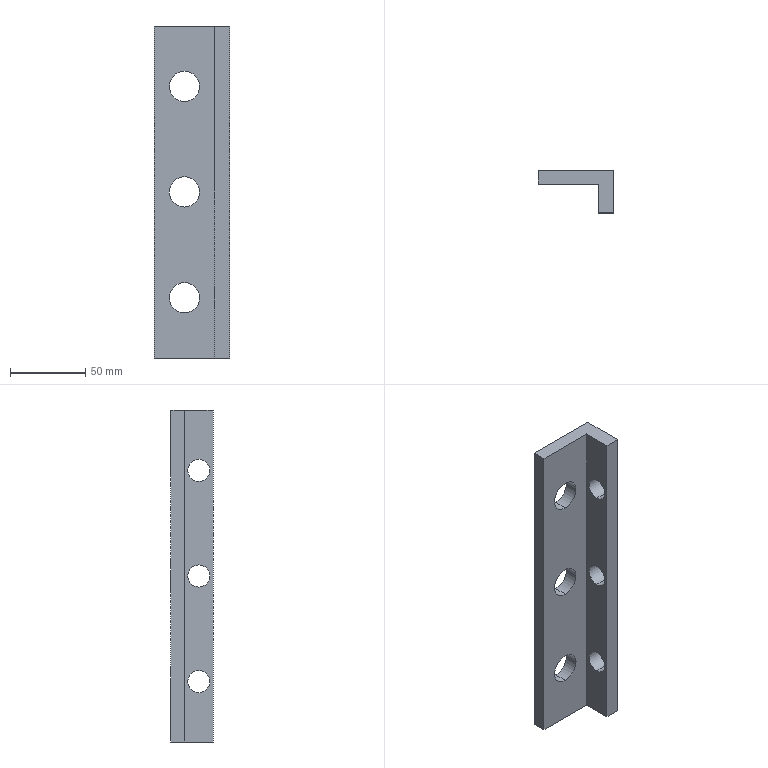Part | SolidWorks | features Cut 4, Extrusion 1 | 1 solid | 29 faces | box 50 x 28 x 220 mm | volume 127251 mm3 | cylinder 21 | plane 8 | commonest cylinder face diameters 20 x15 14.666 x4 14.603 x2
STEP:
#1=CARTESIAN_POINT('',(-15.556,7.75,172.667));
#2=VERTEX_POINT('',#1);
#3=CARTESIAN_POINT('',(-15.556,7.75,187.333));
#4=VERTEX_POINT('',#3);
#5=CARTESIAN_POINT('',(-15.556,7.75,180.));
#6=DIRECTION('',(-1.,0.,0.));
#7=DIRECTION('',(0.,0.,-1.));
#8=AXIS2_PLACEMENT_3D('',#5,#6,#7);
#9=CIRCLE('',#8,7.333);
#10=EDGE_CURVE('',#2,#4,#9,.T.);
#11=ORIENTED_EDGE('',*,*,#10,.T.);
#12=CARTESIAN_POINT('',(-5.556,7.75,187.333));
#13=VERTEX_POINT('',#12);
#14=CARTESIAN_POINT('',(-36.296,7.75,187.333));
#15=DIRECTION('',(1.,0.,0.));
#16=VECTOR('',#15,1000.);
#17=LINE('',#14,#16);
#18=EDGE_CURVE('',#4,#13,#17,.T.);
#19=ORIENTED_EDGE('',*,*,#18,.T.);
#20=CARTESIAN_POINT('',(-5.556,7.75,172.667));
#21=VERTEX_POINT('',#20);
#22=CARTESIAN_POINT('',(-5.556,7.75,180.));
#23=DIRECTION('',(-1.,0.,0.));
#24=DIRECTION('',(0.,-1.,0.));
#25=AXIS2_PLACEMENT_3D('',#22,#23,#24);
#26=CIRCLE('',#25,7.333);
#27=EDGE_CURVE('',#21,#13,#26,.T.);
#28=ORIENTED_EDGE('',*,*,#27,.F.);
#29=CARTESIAN_POINT('',(-36.296,7.75,172.667));
#30=DIRECTION('',(1.,0.,0.));
#31=VECTOR('',#30,1000.);
#32=LINE('',#29,#31);
#33=EDGE_CURVE('',#2,#21,#32,.T.);
#34=ORIENTED_EDGE('',*,*,#33,.F.);
#35=EDGE_LOOP('',(#11,#19,#28,#34));
#36=FACE_OUTER_BOUND('',#35,.T.);
#37=CARTESIAN_POINT('',(-36.296,7.75,180.));
#38=DIRECTION('',(1.,0.,0.));
#39=DIRECTION('',(0.,0.,-1.));
#40=AXIS2_PLACEMENT_3D('',#37,#38,#39);
#41=CYLINDRICAL_SURFACE('',#40,7.333);
#42=ADVANCED_FACE('',(#36),#41,.F.);
#43=CARTESIAN_POINT('',(-5.556,7.75,47.333));
#44=VERTEX_POINT('',#43);
#45=CARTESIAN_POINT('',(-5.556,7.75,32.667));
#46=VERTEX_POINT('',#45);
#47=CARTESIAN_POINT('',(-5.556,7.75,40.));
#48=DIRECTION('',(1.,0.,0.));
#49=DIRECTION('',(0.,-1.,0.));
#50=AXIS2_PLACEMENT_3D('',#47,#48,#49);
#51=CIRCLE('',#50,7.333);
#52=EDGE_CURVE('',#44,#46,#51,.T.);
#53=ORIENTED_EDGE('',*,*,#52,.T.);
#54=CARTESIAN_POINT('',(-15.556,7.75,32.667));
#55=VERTEX_POINT('',#54);
#56=CARTESIAN_POINT('',(15.185,7.75,32.667));
#57=DIRECTION('',(-1.,0.,0.));
#58=VECTOR('',#57,1000.);
#59=LINE('',#56,#58);
#60=EDGE_CURVE('',#46,#55,#59,.T.);
#61=ORIENTED_EDGE('',*,*,#60,.T.);
#62=CARTESIAN_POINT('',(-15.556,7.75,47.333));
#63=VERTEX_POINT('',#62);
#64=CARTESIAN_POINT('',(-15.556,7.75,40.));
#65=DIRECTION('',(-1.,0.,0.));
#66=DIRECTION('',(0.,0.,1.));
#67=AXIS2_PLACEMENT_3D('',#64,#65,#66);
#68=CIRCLE('',#67,7.333);
#69=EDGE_CURVE('',#55,#63,#68,.T.);
#70=ORIENTED_EDGE('',*,*,#69,.T.);
#71=CARTESIAN_POINT('',(15.185,7.75,47.333));
#72=DIRECTION('',(-1.,0.,0.));
#73=VECTOR('',#72,1000.);
#74=LINE('',#71,#73);
#75=EDGE_CURVE('',#44,#63,#74,.T.);
#76=ORIENTED_EDGE('',*,*,#75,.F.);
#77=EDGE_LOOP('',(#53,#61,#70,#76));
#78=FACE_OUTER_BOUND('',#77,.T.);
#79=CARTESIAN_POINT('',(15.185,7.75,40.));
#80=DIRECTION('',(-1.,0.,0.));
#81=DIRECTION('',(0.,0.,1.));
#82=AXIS2_PLACEMENT_3D('',#79,#80,#81);
#83=CYLINDRICAL_SURFACE('',#82,7.333);
#84=ADVANCED_FACE('',(#78),#83,.F.);
#85=CARTESIAN_POINT('',(-5.556,7.75,117.301));
#86=VERTEX_POINT('',#85);
#87=CARTESIAN_POINT('',(-5.556,7.75,102.699));
#88=VERTEX_POINT('',#87);
#89=CARTESIAN_POINT('',(-5.556,7.75,110.));
#90=DIRECTION('',(1.,0.,0.));
#91=DIRECTION('',(0.,-1.,0.));
#92=AXIS2_PLACEMENT_3D('',#89,#90,#91);
#93=CIRCLE('',#92,7.301);
#94=EDGE_CURVE('',#86,#88,#93,.T.);
#95=ORIENTED_EDGE('',*,*,#94,.T.);
#96=CARTESIAN_POINT('',(-15.556,7.75,102.699));
#97=VERTEX_POINT('',#96);
#98=CARTESIAN_POINT('',(15.185,7.75,102.699));
#99=DIRECTION('',(-1.,0.,0.));
#100=VECTOR('',#99,1000.);
#101=LINE('',#98,#100);
#102=EDGE_CURVE('',#88,#97,#101,.T.);
#103=ORIENTED_EDGE('',*,*,#102,.T.);
#104=CARTESIAN_POINT('',(-15.556,7.75,117.301));
#105=VERTEX_POINT('',#104);
#106=CARTESIAN_POINT('',(-15.556,7.75,110.));
#107=DIRECTION('',(-1.,0.,0.));
#108=DIRECTION('',(0.,0.,1.));
#109=AXIS2_PLACEMENT_3D('',#106,#107,#108);
#110=CIRCLE('',#109,7.301);
#111=EDGE_CURVE('',#97,#105,#110,.T.);
#112=ORIENTED_EDGE('',*,*,#111,.T.);
#113=CARTESIAN_POINT('',(15.185,7.75,117.301));
#114=DIRECTION('',(-1.,0.,0.));
#115=VECTOR('',#114,1000.);
#116=LINE('',#113,#115);
#117=EDGE_CURVE('',#86,#105,#116,.T.);
#118=ORIENTED_EDGE('',*,*,#117,.F.);
#119=EDGE_LOOP('',(#95,#103,#112,#118));
#120=FACE_OUTER_BOUND('',#119,.T.);
#121=CARTESIAN_POINT('',(15.185,7.75,110.));
#122=DIRECTION('',(-1.,0.,0.));
#123=DIRECTION('',(0.,0.,1.));
#124=AXIS2_PLACEMENT_3D('',#121,#122,#123);
#125=CYLINDRICAL_SURFACE('',#124,7.301);
#126=ADVANCED_FACE('',(#120),#125,.F.);
#127=CARTESIAN_POINT('',(-35.556,26.25,100.));
#128=VERTEX_POINT('',#127);
#129=CARTESIAN_POINT('',(-25.556,26.25,110.009));
#130=VERTEX_POINT('',#129);
#131=CARTESIAN_POINT('',(-35.556,26.25,110.));
#132=DIRECTION('',(0.,-1.,0.));
#133=DIRECTION('',(0.,0.,-1.));
#134=AXIS2_PLACEMENT_3D('',#131,#132,#133);
#135=CIRCLE('',#134,10.);
#136=EDGE_CURVE('',#128,#130,#135,.T.);
#137=ORIENTED_EDGE('',*,*,#136,.F.);
#138=CARTESIAN_POINT('',(-35.556,17.25,100.));
#139=VERTEX_POINT('',#138);
#140=CARTESIAN_POINT('',(-35.556,69.534,100.));
#141=DIRECTION('',(0.,-1.,0.));
#142=VECTOR('',#141,1000.);
#143=LINE('',#140,#142);
#144=EDGE_CURVE('',#128,#139,#143,.T.);
#145=ORIENTED_EDGE('',*,*,#144,.T.);
#146=CARTESIAN_POINT('',(-25.556,17.25,110.009));
#147=VERTEX_POINT('',#146);
#148=CARTESIAN_POINT('',(-35.556,17.25,110.));
#149=DIRECTION('',(0.,-1.,0.));
#150=DIRECTION('',(0.,0.,-1.));
#151=AXIS2_PLACEMENT_3D('',#148,#149,#150);
#152=CIRCLE('',#151,10.);
#153=EDGE_CURVE('',#139,#147,#152,.T.);
#154=ORIENTED_EDGE('',*,*,#153,.T.);
#155=CARTESIAN_POINT('',(-25.556,29.25,110.009));
#156=DIRECTION('',(0.,-1.,0.));
#157=VECTOR('',#156,1000.);
#158=LINE('',#155,#157);
#159=EDGE_CURVE('',#130,#147,#158,.T.);
#160=ORIENTED_EDGE('',*,*,#159,.F.);
#161=EDGE_LOOP('',(#137,#145,#154,#160));
#162=FACE_OUTER_BOUND('',#161,.T.);
#163=CARTESIAN_POINT('',(-35.556,69.534,110.));
#164=DIRECTION('',(0.,-1.,0.));
#165=DIRECTION('',(0.,0.,-1.));
#166=AXIS2_PLACEMENT_3D('',#163,#164,#165);
#167=CYLINDRICAL_SURFACE('',#166,10.);
#168=ADVANCED_FACE('',(#162),#167,.F.);
#169=CARTESIAN_POINT('',(-35.556,26.25,29.982));
#170=VERTEX_POINT('',#169);
#171=CARTESIAN_POINT('',(-25.556,26.25,39.991));
#172=VERTEX_POINT('',#171);
#173=CARTESIAN_POINT('',(-35.556,26.25,39.982));
#174=DIRECTION('',(0.,-1.,0.));
#175=DIRECTION('',(0.,0.,-1.));
#176=AXIS2_PLACEMENT_3D('',#173,#174,#175);
#177=CIRCLE('',#176,10.);
#178=EDGE_CURVE('',#170,#172,#177,.T.);
#179=ORIENTED_EDGE('',*,*,#178,.F.);
#180=CARTESIAN_POINT('',(-35.556,17.25,29.982));
#181=VERTEX_POINT('',#180);
#182=CARTESIAN_POINT('',(-35.556,69.534,29.982));
#183=DIRECTION('',(0.,-1.,0.));
#184=VECTOR('',#183,1000.);
#185=LINE('',#182,#184);
#186=EDGE_CURVE('',#170,#181,#185,.T.);
#187=ORIENTED_EDGE('',*,*,#186,.T.);
#188=CARTESIAN_POINT('',(-25.556,17.25,39.991));
#189=VERTEX_POINT('',#188);
#190=CARTESIAN_POINT('',(-35.556,17.25,39.982));
#191=DIRECTION('',(0.,-1.,0.));
#192=DIRECTION('',(0.,0.,-1.));
#193=AXIS2_PLACEMENT_3D('',#190,#191,#192);
#194=CIRCLE('',#193,10.);
#195=EDGE_CURVE('',#181,#189,#194,.T.);
#196=ORIENTED_EDGE('',*,*,#195,.T.);
#197=CARTESIAN_POINT('',(-25.556,29.25,39.991));
#198=DIRECTION('',(0.,-1.,0.));
#199=VECTOR('',#198,1000.);
#200=LINE('',#197,#199);
#201=EDGE_CURVE('',#172,#189,#200,.T.);
#202=ORIENTED_EDGE('',*,*,#201,.F.);
#203=EDGE_LOOP('',(#179,#187,#196,#202));
#204=FACE_OUTER_BOUND('',#203,.T.);
#205=CARTESIAN_POINT('',(-35.556,69.534,39.982));
#206=DIRECTION('',(0.,-1.,0.));
#207=DIRECTION('',(0.,0.,-1.));
#208=AXIS2_PLACEMENT_3D('',#205,#206,#207);
#209=CYLINDRICAL_SURFACE('',#208,10.);
#210=ADVANCED_FACE('',(#204),#209,.F.);
#211=CARTESIAN_POINT('',(-35.556,26.25,170.));
#212=VERTEX_POINT('',#211);
#213=CARTESIAN_POINT('',(-25.556,26.25,180.018));
#214=VERTEX_POINT('',#213);
#215=CARTESIAN_POINT('',(-35.556,26.25,180.));
#216=DIRECTION('',(0.,-1.,0.));
#217=DIRECTION('',(0.,0.,-1.));
#218=AXIS2_PLACEMENT_3D('',#215,#216,#217);
#219=CIRCLE('',#218,10.);
#220=EDGE_CURVE('',#212,#214,#219,.T.);
#221=ORIENTED_EDGE('',*,*,#220,.F.);
#222=CARTESIAN_POINT('',(-35.556,17.25,170.));
#223=VERTEX_POINT('',#222);
#224=CARTESIAN_POINT('',(-35.556,69.534,170.));
#225=DIRECTION('',(0.,-1.,0.));
#226=VECTOR('',#225,1000.);
#227=LINE('',#224,#226);
#228=EDGE_CURVE('',#212,#223,#227,.T.);
#229=ORIENTED_EDGE('',*,*,#228,.T.);
#230=CARTESIAN_POINT('',(-25.556,17.25,180.018));
#231=VERTEX_POINT('',#230);
#232=CARTESIAN_POINT('',(-35.556,17.25,180.));
#233=DIRECTION('',(0.,-1.,0.));
#234=DIRECTION('',(0.,0.,-1.));
#235=AXIS2_PLACEMENT_3D('',#232,#233,#234);
#236=CIRCLE('',#235,10.);
#237=EDGE_CURVE('',#223,#231,#236,.T.);
#238=ORIENTED_EDGE('',*,*,#237,.T.);
#239=CARTESIAN_POINT('',(-25.556,29.25,180.018));
#240=DIRECTION('',(0.,-1.,0.));
#241=VECTOR('',#240,1000.);
#242=LINE('',#239,#241);
#243=EDGE_CURVE('',#214,#231,#242,.T.);
#244=ORIENTED_EDGE('',*,*,#243,.F.);
#245=EDGE_LOOP('',(#221,#229,#238,#244));
#246=FACE_OUTER_BOUND('',#245,.T.);
#247=CARTESIAN_POINT('',(-35.556,69.534,180.));
#248=DIRECTION('',(0.,-1.,0.));
#249=DIRECTION('',(0.,0.,-1.));
#250=AXIS2_PLACEMENT_3D('',#247,#248,#249);
#251=CYLINDRICAL_SURFACE('',#250,10.);
#252=ADVANCED_FACE('',(#246),#251,.F.);
#253=CARTESIAN_POINT('',(-45.556,26.25,180.036));
#254=VERTEX_POINT('',#253);
#255=CARTESIAN_POINT('',(-45.556,26.25,180.018));
#256=VERTEX_POINT('',#255);
#257=CARTESIAN_POINT('',(-35.556,26.25,180.036));
#258=DIRECTION('',(0.,-1.,0.));
#259=DIRECTION('',(0.,0.,-1.));
#260=AXIS2_PLACEMENT_3D('',#257,#258,#259);
#261=CIRCLE('',#260,10.);
#262=EDGE_CURVE('',#254,#256,#261,.T.);
#263=ORIENTED_EDGE('',*,*,#262,.F.);
#264=CARTESIAN_POINT('',(-45.556,17.25,180.036));
#265=VERTEX_POINT('',#264);
#266=CARTESIAN_POINT('',(-45.556,69.534,180.036));
#267=DIRECTION('',(0.,-1.,0.));
#268=VECTOR('',#267,1000.);
#269=LINE('',#266,#268);
#270=EDGE_CURVE('',#254,#265,#269,.T.);
#271=ORIENTED_EDGE('',*,*,#270,.T.);
#272=CARTESIAN_POINT('',(-45.556,17.25,180.018));
#273=VERTEX_POINT('',#272);
#274=CARTESIAN_POINT('',(-35.556,17.25,180.036));
#275=DIRECTION('',(0.,-1.,0.));
#276=DIRECTION('',(1.,0.,0.));
#277=AXIS2_PLACEMENT_3D('',#274,#275,#276);
#278=CIRCLE('',#277,10.);
#279=EDGE_CURVE('',#265,#273,#278,.T.);
#280=ORIENTED_EDGE('',*,*,#279,.T.);
#281=CARTESIAN_POINT('',(-45.556,29.25,180.018));
#282=DIRECTION('',(0.,1.,0.));
#283=VECTOR('',#282,1000.);
#284=LINE('',#281,#283);
#285=EDGE_CURVE('',#273,#256,#284,.T.);
#286=ORIENTED_EDGE('',*,*,#285,.T.);
#287=EDGE_LOOP('',(#263,#271,#280,#286));
#288=FACE_OUTER_BOUND('',#287,.T.);
#289=CARTESIAN_POINT('',(-35.556,69.534,180.036));
#290=DIRECTION('',(0.,-1.,0.));
#291=DIRECTION('',(1.,0.,0.));
#292=AXIS2_PLACEMENT_3D('',#289,#290,#291);
#293=CYLINDRICAL_SURFACE('',#292,10.);
#294=ADVANCED_FACE('',(#288),#293,.F.);
#295=ORIENTED_EDGE('',*,*,#270,.F.);
#296=CARTESIAN_POINT('',(-25.556,26.25,180.036));
#297=VERTEX_POINT('',#296);
#298=CARTESIAN_POINT('',(-35.556,26.25,180.036));
#299=DIRECTION('',(0.,-1.,0.));
#300=DIRECTION('',(0.,0.,-1.));
#301=AXIS2_PLACEMENT_3D('',#298,#299,#300);
#302=CIRCLE('',#301,10.);
#303=EDGE_CURVE('',#297,#254,#302,.T.);
#304=ORIENTED_EDGE('',*,*,#303,.F.);
#305=CARTESIAN_POINT('',(-25.556,17.25,180.036));
#306=VERTEX_POINT('',#305);
#307=CARTESIAN_POINT('',(-25.556,69.534,180.036));
#308=DIRECTION('',(0.,-1.,0.));
#309=VECTOR('',#308,1000.);
#310=LINE('',#307,#309);
#311=EDGE_CURVE('',#297,#306,#310,.T.);
#312=ORIENTED_EDGE('',*,*,#311,.T.);
#313=CARTESIAN_POINT('',(-35.556,17.25,180.036));
#314=DIRECTION('',(0.,-1.,0.));
#315=DIRECTION('',(1.,0.,0.));
#316=AXIS2_PLACEMENT_3D('',#313,#314,#315);
#317=CIRCLE('',#316,10.);
#318=EDGE_CURVE('',#306,#265,#317,.T.);
#319=ORIENTED_EDGE('',*,*,#318,.T.);
#320=EDGE_LOOP('',(#295,#304,#312,#319));
#321=FACE_OUTER_BOUND('',#320,.T.);
#322=CARTESIAN_POINT('',(-35.556,69.534,180.036));
#323=DIRECTION('',(0.,-1.,0.));
#324=DIRECTION('',(1.,0.,0.));
#325=AXIS2_PLACEMENT_3D('',#322,#323,#324);
#326=CYLINDRICAL_SURFACE('',#325,10.);
#327=ADVANCED_FACE('',(#321),#326,.F.);
#328=CARTESIAN_POINT('',(-45.556,26.25,40.));
#329=VERTEX_POINT('',#328);
#330=CARTESIAN_POINT('',(-45.556,26.25,39.991));
#331=VERTEX_POINT('',#330);
#332=CARTESIAN_POINT('',(-35.556,26.25,40.));
#333=DIRECTION('',(0.,-1.,0.));
#334=DIRECTION('',(0.,0.,-1.));
#335=AXIS2_PLACEMENT_3D('',#332,#333,#334);
#336=CIRCLE('',#335,10.);
#337=EDGE_CURVE('',#329,#331,#336,.T.);
#338=ORIENTED_EDGE('',*,*,#337,.F.);
#339=CARTESIAN_POINT('',(-45.556,17.25,40.));
#340=VERTEX_POINT('',#339);
#341=CARTESIAN_POINT('',(-45.556,69.534,40.));
#342=DIRECTION('',(0.,-1.,0.));
#343=VECTOR('',#342,1000.);
#344=LINE('',#341,#343);
#345=EDGE_CURVE('',#329,#340,#344,.T.);
#346=ORIENTED_EDGE('',*,*,#345,.T.);
#347=CARTESIAN_POINT('',(-45.556,17.25,39.991));
#348=VERTEX_POINT('',#347);
#349=CARTESIAN_POINT('',(-35.556,17.25,40.));
#350=DIRECTION('',(0.,-1.,0.));
#351=DIRECTION('',(1.,0.,0.));
#352=AXIS2_PLACEMENT_3D('',#349,#350,#351);
#353=CIRCLE('',#352,10.);
#354=EDGE_CURVE('',#340,#348,#353,.T.);
#355=ORIENTED_EDGE('',*,*,#354,.T.);
#356=CARTESIAN_POINT('',(-45.556,29.25,39.991));
#357=DIRECTION('',(0.,1.,0.));
#358=VECTOR('',#357,1000.);
#359=LINE('',#356,#358);
#360=EDGE_CURVE('',#348,#331,#359,.T.);
#361=ORIENTED_EDGE('',*,*,#360,.T.);
#362=EDGE_LOOP('',(#338,#346,#355,#361));
#363=FACE_OUTER_BOUND('',#362,.T.);
#364=CARTESIAN_POINT('',(-35.556,69.534,40.));
#365=DIRECTION('',(0.,-1.,0.));
#366=DIRECTION('',(1.,0.,0.));
#367=AXIS2_PLACEMENT_3D('',#364,#365,#366);
#368=CYLINDRICAL_SURFACE('',#367,10.);
#369=ADVANCED_FACE('',(#363),#368,.F.);
#370=ORIENTED_EDGE('',*,*,#345,.F.);
#371=CARTESIAN_POINT('',(-25.556,26.25,40.));
#372=VERTEX_POINT('',#371);
#373=CARTESIAN_POINT('',(-35.556,26.25,40.));
#374=DIRECTION('',(0.,-1.,0.));
#375=DIRECTION('',(0.,0.,-1.));
#376=AXIS2_PLACEMENT_3D('',#373,#374,#375);
#377=CIRCLE('',#376,10.);
#378=EDGE_CURVE('',#372,#329,#377,.T.);
#379=ORIENTED_EDGE('',*,*,#378,.F.);
#380=CARTESIAN_POINT('',(-25.556,17.25,40.));
#381=VERTEX_POINT('',#380);
#382=CARTESIAN_POINT('',(-25.556,69.534,40.));
#383=DIRECTION('',(0.,-1.,0.));
#384=VECTOR('',#383,1000.);
#385=LINE('',#382,#384);
#386=EDGE_CURVE('',#372,#381,#385,.T.);
#387=ORIENTED_EDGE('',*,*,#386,.T.);
#388=CARTESIAN_POINT('',(-35.556,17.25,40.));
#389=DIRECTION('',(0.,-1.,0.));
#390=DIRECTION('',(1.,0.,0.));
#391=AXIS2_PLACEMENT_3D('',#388,#389,#390);
#392=CIRCLE('',#391,10.);
#393=EDGE_CURVE('',#381,#340,#392,.T.);
#394=ORIENTED_EDGE('',*,*,#393,.T.);
#395=EDGE_LOOP('',(#370,#379,#387,#394));
#396=FACE_OUTER_BOUND('',#395,.T.);
#397=CARTESIAN_POINT('',(-35.556,69.534,40.));
#398=DIRECTION('',(0.,-1.,0.));
#399=DIRECTION('',(1.,0.,0.));
#400=AXIS2_PLACEMENT_3D('',#397,#398,#399);
#401=CYLINDRICAL_SURFACE('',#400,10.);
#402=ADVANCED_FACE('',(#396),#401,.F.);
#403=CARTESIAN_POINT('',(-45.556,26.25,110.018));
#404=VERTEX_POINT('',#403);
#405=CARTESIAN_POINT('',(-45.556,26.25,110.009));
#406=VERTEX_POINT('',#405);
#407=CARTESIAN_POINT('',(-35.556,26.25,110.018));
#408=DIRECTION('',(0.,-1.,0.));
#409=DIRECTION('',(0.,0.,-1.));
#410=AXIS2_PLACEMENT_3D('',#407,#408,#409);
#411=CIRCLE('',#410,10.);
#412=EDGE_CURVE('',#404,#406,#411,.T.);
#413=ORIENTED_EDGE('',*,*,#412,.F.);
#414=CARTESIAN_POINT('',(-45.556,17.25,110.018));
#415=VERTEX_POINT('',#414);
#416=CARTESIAN_POINT('',(-45.556,69.534,110.018));
#417=DIRECTION('',(0.,-1.,0.));
#418=VECTOR('',#417,1000.);
#419=LINE('',#416,#418);
#420=EDGE_CURVE('',#404,#415,#419,.T.);
#421=ORIENTED_EDGE('',*,*,#420,.T.);
#422=CARTESIAN_POINT('',(-45.556,17.25,110.009));
#423=VERTEX_POINT('',#422);
#424=CARTESIAN_POINT('',(-35.556,17.25,110.018));
#425=DIRECTION('',(0.,-1.,0.));
#426=DIRECTION('',(1.,0.,0.));
#427=AXIS2_PLACEMENT_3D('',#424,#425,#426);
#428=CIRCLE('',#427,10.);
#429=EDGE_CURVE('',#415,#423,#428,.T.);
#430=ORIENTED_EDGE('',*,*,#429,.T.);
#431=CARTESIAN_POINT('',(-45.556,29.25,110.009));
#432=DIRECTION('',(0.,1.,0.));
#433=VECTOR('',#432,1000.);
#434=LINE('',#431,#433);
#435=EDGE_CURVE('',#423,#406,#434,.T.);
#436=ORIENTED_EDGE('',*,*,#435,.T.);
#437=EDGE_LOOP('',(#413,#421,#430,#436));
#438=FACE_OUTER_BOUND('',#437,.T.);
#439=CARTESIAN_POINT('',(-35.556,69.534,110.018));
#440=DIRECTION('',(0.,-1.,0.));
#441=DIRECTION('',(1.,0.,0.));
#442=AXIS2_PLACEMENT_3D('',#439,#440,#441);
#443=CYLINDRICAL_SURFACE('',#442,10.);
#444=ADVANCED_FACE('',(#438),#443,.F.);
#445=ORIENTED_EDGE('',*,*,#420,.F.);
#446=CARTESIAN_POINT('',(-25.556,26.25,110.018));
#447=VERTEX_POINT('',#446);
#448=CARTESIAN_POINT('',(-35.556,26.25,110.018));
#449=DIRECTION('',(0.,-1.,0.));
#450=DIRECTION('',(0.,0.,-1.));
#451=AXIS2_PLACEMENT_3D('',#448,#449,#450);
#452=CIRCLE('',#451,10.);
#453=EDGE_CURVE('',#447,#404,#452,.T.);
#454=ORIENTED_EDGE('',*,*,#453,.F.);
#455=CARTESIAN_POINT('',(-25.556,17.25,110.018));
#456=VERTEX_POINT('',#455);
#457=CARTESIAN_POINT('',(-25.556,69.534,110.018));
#458=DIRECTION('',(0.,-1.,0.));
#459=VECTOR('',#458,1000.);
#460=LINE('',#457,#459);
#461=EDGE_CURVE('',#447,#456,#460,.T.);
#462=ORIENTED_EDGE('',*,*,#461,.T.);
#463=CARTESIAN_POINT('',(-35.556,17.25,110.018));
#464=DIRECTION('',(0.,-1.,0.));
#465=DIRECTION('',(1.,0.,0.));
#466=AXIS2_PLACEMENT_3D('',#463,#464,#465);
#467=CIRCLE('',#466,10.);
#468=EDGE_CURVE('',#456,#415,#467,.T.);
#469=ORIENTED_EDGE('',*,*,#468,.T.);
#470=EDGE_LOOP('',(#445,#454,#462,#469));
#471=FACE_OUTER_BOUND('',#470,.T.);
#472=CARTESIAN_POINT('',(-35.556,69.534,110.018));
#473=DIRECTION('',(0.,-1.,0.));
#474=DIRECTION('',(1.,0.,0.));
#475=AXIS2_PLACEMENT_3D('',#472,#473,#474);
#476=CYLINDRICAL_SURFACE('',#475,10.);
#477=ADVANCED_FACE('',(#471),#476,.F.);
#478=CARTESIAN_POINT('',(-55.556,26.25,0.));
#479=VERTEX_POINT('',#478);
#480=CARTESIAN_POINT('',(-55.556,17.25,0.));
#481=VERTEX_POINT('',#480);
#482=CARTESIAN_POINT('',(-55.556,26.25,0.));
#483=DIRECTION('',(0.,-1.,0.));
#484=VECTOR('',#483,1000.);
#485=LINE('',#482,#484);
#486=EDGE_CURVE('',#479,#481,#485,.T.);
#487=ORIENTED_EDGE('',*,*,#486,.T.);
#488=CARTESIAN_POINT('',(-55.556,17.25,220.));
#489=VERTEX_POINT('',#488);
#490=CARTESIAN_POINT('',(-55.556,17.25,220.));
#491=DIRECTION('',(0.,0.,-1.));
#492=VECTOR('',#491,1000.);
#493=LINE('',#490,#492);
#494=EDGE_CURVE('',#489,#481,#493,.T.);
#495=ORIENTED_EDGE('',*,*,#494,.F.);
#496=CARTESIAN_POINT('',(-55.556,26.25,220.));
#497=VERTEX_POINT('',#496);
#498=CARTESIAN_POINT('',(-55.556,26.25,220.));
#499=DIRECTION('',(0.,-1.,0.));
#500=VECTOR('',#499,1000.);
#501=LINE('',#498,#500);
#502=EDGE_CURVE('',#497,#489,#501,.T.);
#503=ORIENTED_EDGE('',*,*,#502,.F.);
#504=CARTESIAN_POINT('',(-55.556,26.25,220.));
#505=DIRECTION('',(0.,0.,-1.));
#506=VECTOR('',#505,1000.);
#507=LINE('',#504,#506);
#508=EDGE_CURVE('',#497,#479,#507,.T.);
#509=ORIENTED_EDGE('',*,*,#508,.T.);
#510=EDGE_LOOP('',(#487,#495,#503,#509));
#511=FACE_OUTER_BOUND('',#510,.T.);
#512=CARTESIAN_POINT('',(-55.556,26.25,220.));
#513=DIRECTION('',(1.,0.,0.));
#514=DIRECTION('',(0.,0.,-1.));
#515=AXIS2_PLACEMENT_3D('',#512,#513,#514);
#516=PLANE('',#515);
#517=ADVANCED_FACE('',(#511),#516,.F.);
#518=CARTESIAN_POINT('',(-35.556,17.25,180.036));
#519=DIRECTION('',(0.,-1.,0.));
#520=DIRECTION('',(1.,0.,0.));
#521=AXIS2_PLACEMENT_3D('',#518,#519,#520);
#522=CIRCLE('',#521,10.);
#523=EDGE_CURVE('',#231,#306,#522,.T.);
#524=ORIENTED_EDGE('',*,*,#523,.F.);
#525=ORIENTED_EDGE('',*,*,#237,.F.);
#526=CARTESIAN_POINT('',(-35.556,17.25,180.));
#527=DIRECTION('',(0.,-1.,0.));
#528=DIRECTION('',(0.,0.,-1.));
#529=AXIS2_PLACEMENT_3D('',#526,#527,#528);
#530=CIRCLE('',#529,10.);
#531=EDGE_CURVE('',#273,#223,#530,.T.);
#532=ORIENTED_EDGE('',*,*,#531,.F.);
#533=ORIENTED_EDGE('',*,*,#279,.F.);
#534=ORIENTED_EDGE('',*,*,#318,.F.);
#535=EDGE_LOOP('',(#524,#525,#532,#533,#534));
#536=FACE_BOUND('',#535,.T.);
#537=CARTESIAN_POINT('',(-35.556,17.25,40.));
#538=DIRECTION('',(0.,-1.,0.));
#539=DIRECTION('',(1.,0.,0.));
#540=AXIS2_PLACEMENT_3D('',#537,#538,#539);
#541=CIRCLE('',#540,10.);
#542=EDGE_CURVE('',#189,#381,#541,.T.);
#543=ORIENTED_EDGE('',*,*,#542,.F.);
#544=ORIENTED_EDGE('',*,*,#195,.F.);
#545=CARTESIAN_POINT('',(-35.556,17.25,39.982));
#546=DIRECTION('',(0.,-1.,0.));
#547=DIRECTION('',(0.,0.,-1.));
#548=AXIS2_PLACEMENT_3D('',#545,#546,#547);
#549=CIRCLE('',#548,10.);
#550=EDGE_CURVE('',#348,#181,#549,.T.);
#551=ORIENTED_EDGE('',*,*,#550,.F.);
#552=ORIENTED_EDGE('',*,*,#354,.F.);
#553=ORIENTED_EDGE('',*,*,#393,.F.);
#554=EDGE_LOOP('',(#543,#544,#551,#552,#553));
#555=FACE_BOUND('',#554,.T.);
#556=CARTESIAN_POINT('',(-35.556,17.25,110.018));
#557=DIRECTION('',(0.,-1.,0.));
#558=DIRECTION('',(1.,0.,0.));
#559=AXIS2_PLACEMENT_3D('',#556,#557,#558);
#560=CIRCLE('',#559,10.);
#561=EDGE_CURVE('',#147,#456,#560,.T.);
#562=ORIENTED_EDGE('',*,*,#561,.F.);
#563=ORIENTED_EDGE('',*,*,#153,.F.);
#564=CARTESIAN_POINT('',(-35.556,17.25,110.));
#565=DIRECTION('',(0.,-1.,0.));
#566=DIRECTION('',(0.,0.,-1.));
#567=AXIS2_PLACEMENT_3D('',#564,#565,#566);
#568=CIRCLE('',#567,10.);
#569=EDGE_CURVE('',#423,#139,#568,.T.);
#570=ORIENTED_EDGE('',*,*,#569,.F.);
#571=ORIENTED_EDGE('',*,*,#429,.F.);
#572=ORIENTED_EDGE('',*,*,#468,.F.);
#573=EDGE_LOOP('',(#562,#563,#570,#571,#572));
#574=FACE_BOUND('',#573,.T.);
#575=CARTESIAN_POINT('',(-15.556,17.25,0.));
#576=VERTEX_POINT('',#575);
#577=CARTESIAN_POINT('',(-15.556,17.25,0.));
#578=DIRECTION('',(1.,0.,0.));
#579=VECTOR('',#578,1000.);
#580=LINE('',#577,#579);
#581=EDGE_CURVE('',#481,#576,#580,.T.);
#582=ORIENTED_EDGE('',*,*,#581,.T.);
#583=CARTESIAN_POINT('',(-15.556,17.25,220.));
#584=VERTEX_POINT('',#583);
#585=CARTESIAN_POINT('',(-15.556,17.25,220.));
#586=DIRECTION('',(0.,0.,-1.));
#587=VECTOR('',#586,1000.);
#588=LINE('',#585,#587);
#589=EDGE_CURVE('',#584,#576,#588,.T.);
#590=ORIENTED_EDGE('',*,*,#589,.F.);
#591=CARTESIAN_POINT('',(-15.556,17.25,220.));
#592=DIRECTION('',(1.,0.,0.));
#593=VECTOR('',#592,1000.);
#594=LINE('',#591,#593);
#595=EDGE_CURVE('',#489,#584,#594,.T.);
#596=ORIENTED_EDGE('',*,*,#595,.F.);
#597=ORIENTED_EDGE('',*,*,#494,.T.);
#598=EDGE_LOOP('',(#582,#590,#596,#597));
#599=FACE_OUTER_BOUND('',#598,.T.);
#600=CARTESIAN_POINT('',(-15.556,17.25,220.));
#601=DIRECTION('',(0.,1.,0.));
#602=DIRECTION('',(-1.,0.,0.));
#603=AXIS2_PLACEMENT_3D('',#600,#601,#602);
#604=PLANE('',#603);
#605=ADVANCED_FACE('',(#536,#555,#574,#599),#604,.F.);
#606=ORIENTED_EDGE('',*,*,#10,.F.);
#607=CARTESIAN_POINT('',(-15.556,7.75,180.));
#608=DIRECTION('',(-1.,0.,0.));
#609=DIRECTION('',(0.,0.,-1.));
#610=AXIS2_PLACEMENT_3D('',#607,#608,#609);
#611=CIRCLE('',#610,7.333);
#612=EDGE_CURVE('',#4,#2,#611,.T.);
#613=ORIENTED_EDGE('',*,*,#612,.F.);
#614=EDGE_LOOP('',(#606,#613));
#615=FACE_BOUND('',#614,.T.);
#616=CARTESIAN_POINT('',(-15.556,7.75,40.));
#617=DIRECTION('',(-1.,0.,0.));
#618=DIRECTION('',(0.,0.,1.));
#619=AXIS2_PLACEMENT_3D('',#616,#617,#618);
#620=CIRCLE('',#619,7.333);
#621=EDGE_CURVE('',#63,#55,#620,.T.);
#622=ORIENTED_EDGE('',*,*,#621,.F.);
#623=ORIENTED_EDGE('',*,*,#69,.F.);
#624=EDGE_LOOP('',(#622,#623));
#625=FACE_BOUND('',#624,.T.);
#626=CARTESIAN_POINT('',(-15.556,7.75,110.));
#627=DIRECTION('',(-1.,0.,0.));
#628=DIRECTION('',(0.,0.,1.));
#629=AXIS2_PLACEMENT_3D('',#626,#627,#628);
#630=CIRCLE('',#629,7.301);
#631=EDGE_CURVE('',#105,#97,#630,.T.);
#632=ORIENTED_EDGE('',*,*,#631,.F.);
#633=ORIENTED_EDGE('',*,*,#111,.F.);
#634=EDGE_LOOP('',(#632,#633));
#635=FACE_BOUND('',#634,.T.);
#636=CARTESIAN_POINT('',(-15.556,-1.75,0.));
#637=VERTEX_POINT('',#636);
#638=CARTESIAN_POINT('',(-15.556,-1.75,0.));
#639=DIRECTION('',(0.,-1.,0.));
#640=VECTOR('',#639,1000.);
#641=LINE('',#638,#640);
#642=EDGE_CURVE('',#576,#637,#641,.T.);
#643=ORIENTED_EDGE('',*,*,#642,.T.);
#644=CARTESIAN_POINT('',(-15.556,-1.75,220.));
#645=VERTEX_POINT('',#644);
#646=CARTESIAN_POINT('',(-15.556,-1.75,220.));
#647=DIRECTION('',(0.,0.,-1.));
#648=VECTOR('',#647,1000.);
#649=LINE('',#646,#648);
#650=EDGE_CURVE('',#645,#637,#649,.T.);
#651=ORIENTED_EDGE('',*,*,#650,.F.);
#652=CARTESIAN_POINT('',(-15.556,-1.75,220.));
#653=DIRECTION('',(0.,-1.,0.));
#654=VECTOR('',#653,1000.);
#655=LINE('',#652,#654);
#656=EDGE_CURVE('',#584,#645,#655,.T.);
#657=ORIENTED_EDGE('',*,*,#656,.F.);
#658=ORIENTED_EDGE('',*,*,#589,.T.);
#659=EDGE_LOOP('',(#643,#651,#657,#658));
#660=FACE_OUTER_BOUND('',#659,.T.);
#661=CARTESIAN_POINT('',(-15.556,-1.75,220.));
#662=DIRECTION('',(1.,0.,0.));
#663=DIRECTION('',(0.,0.,-1.));
#664=AXIS2_PLACEMENT_3D('',#661,#662,#663);
#665=PLANE('',#664);
#666=ADVANCED_FACE('',(#615,#625,#635,#660),#665,.F.);
#667=CARTESIAN_POINT('',(-5.556,-1.75,0.));
#668=VERTEX_POINT('',#667);
#669=CARTESIAN_POINT('',(-5.556,-1.75,0.));
#670=DIRECTION('',(1.,0.,0.));
#671=VECTOR('',#670,1000.);
#672=LINE('',#669,#671);
#673=EDGE_CURVE('',#637,#668,#672,.T.);
#674=ORIENTED_EDGE('',*,*,#673,.T.);
#675=CARTESIAN_POINT('',(-5.556,-1.75,220.));
#676=VERTEX_POINT('',#675);
#677=CARTESIAN_POINT('',(-5.556,-1.75,220.));
#678=DIRECTION('',(0.,0.,-1.));
#679=VECTOR('',#678,1000.);
#680=LINE('',#677,#679);
#681=EDGE_CURVE('',#676,#668,#680,.T.);
#682=ORIENTED_EDGE('',*,*,#681,.F.);
#683=CARTESIAN_POINT('',(-5.556,-1.75,220.));
#684=DIRECTION('',(1.,0.,0.));
#685=VECTOR('',#684,1000.);
#686=LINE('',#683,#685);
#687=EDGE_CURVE('',#645,#676,#686,.T.);
#688=ORIENTED_EDGE('',*,*,#687,.F.);
#689=ORIENTED_EDGE('',*,*,#650,.T.);
#690=EDGE_LOOP('',(#674,#682,#688,#689));
#691=FACE_OUTER_BOUND('',#690,.T.);
#692=CARTESIAN_POINT('',(-5.556,-1.75,220.));
#693=DIRECTION('',(0.,1.,0.));
#694=DIRECTION('',(0.,0.,1.));
#695=AXIS2_PLACEMENT_3D('',#692,#693,#694);
#696=PLANE('',#695);
#697=ADVANCED_FACE('',(#691),#696,.F.);
#698=ORIENTED_EDGE('',*,*,#27,.T.);
#699=CARTESIAN_POINT('',(-5.556,7.75,180.));
#700=DIRECTION('',(-1.,0.,0.));
#701=DIRECTION('',(0.,-1.,0.));
#702=AXIS2_PLACEMENT_3D('',#699,#700,#701);
#703=CIRCLE('',#702,7.333);
#704=EDGE_CURVE('',#13,#21,#703,.T.);
#705=ORIENTED_EDGE('',*,*,#704,.T.);
#706=EDGE_LOOP('',(#698,#705));
#707=FACE_BOUND('',#706,.T.);
#708=ORIENTED_EDGE('',*,*,#52,.F.);
#709=CARTESIAN_POINT('',(-5.556,7.75,40.));
#710=DIRECTION('',(1.,0.,0.));
#711=DIRECTION('',(0.,-1.,0.));
#712=AXIS2_PLACEMENT_3D('',#709,#710,#711);
#713=CIRCLE('',#712,7.333);
#714=EDGE_CURVE('',#46,#44,#713,.T.);
#715=ORIENTED_EDGE('',*,*,#714,.F.);
#716=EDGE_LOOP('',(#708,#715));
#717=FACE_BOUND('',#716,.T.);
#718=ORIENTED_EDGE('',*,*,#94,.F.);
#719=CARTESIAN_POINT('',(-5.556,7.75,110.));
#720=DIRECTION('',(1.,0.,0.));
#721=DIRECTION('',(0.,-1.,0.));
#722=AXIS2_PLACEMENT_3D('',#719,#720,#721);
#723=CIRCLE('',#722,7.301);
#724=EDGE_CURVE('',#88,#86,#723,.T.);
#725=ORIENTED_EDGE('',*,*,#724,.F.);
#726=EDGE_LOOP('',(#718,#725));
#727=FACE_BOUND('',#726,.T.);
#728=CARTESIAN_POINT('',(-5.556,26.25,0.));
#729=VERTEX_POINT('',#728);
#730=CARTESIAN_POINT('',(-5.556,26.25,0.));
#731=DIRECTION('',(0.,1.,0.));
#732=VECTOR('',#731,1000.);
#733=LINE('',#730,#732);
#734=EDGE_CURVE('',#668,#729,#733,.T.);
#735=ORIENTED_EDGE('',*,*,#734,.T.);
#736=CARTESIAN_POINT('',(-5.556,26.25,220.));
#737=VERTEX_POINT('',#736);
#738=CARTESIAN_POINT('',(-5.556,26.25,220.));
#739=DIRECTION('',(0.,0.,-1.));
#740=VECTOR('',#739,1000.);
#741=LINE('',#738,#740);
#742=EDGE_CURVE('',#737,#729,#741,.T.);
#743=ORIENTED_EDGE('',*,*,#742,.F.);
#744=CARTESIAN_POINT('',(-5.556,26.25,220.));
#745=DIRECTION('',(0.,1.,0.));
#746=VECTOR('',#745,1000.);
#747=LINE('',#744,#746);
#748=EDGE_CURVE('',#676,#737,#747,.T.);
#749=ORIENTED_EDGE('',*,*,#748,.F.);
#750=ORIENTED_EDGE('',*,*,#681,.T.);
#751=EDGE_LOOP('',(#735,#743,#749,#750));
#752=FACE_OUTER_BOUND('',#751,.T.);
#753=CARTESIAN_POINT('',(-5.556,26.25,220.));
#754=DIRECTION('',(-1.,0.,0.));
#755=DIRECTION('',(0.,-1.,0.));
#756=AXIS2_PLACEMENT_3D('',#753,#754,#755);
#757=PLANE('',#756);
#758=ADVANCED_FACE('',(#707,#717,#727,#752),#757,.F.);
#759=CARTESIAN_POINT('',(-35.556,26.25,180.036));
#760=DIRECTION('',(0.,-1.,0.));
#761=DIRECTION('',(0.,0.,-1.));
#762=AXIS2_PLACEMENT_3D('',#759,#760,#761);
#763=CIRCLE('',#762,10.);
#764=EDGE_CURVE('',#214,#297,#763,.T.);
#765=ORIENTED_EDGE('',*,*,#764,.T.);
#766=ORIENTED_EDGE('',*,*,#303,.T.);
#767=ORIENTED_EDGE('',*,*,#262,.T.);
#768=CARTESIAN_POINT('',(-35.556,26.25,180.));
#769=DIRECTION('',(0.,-1.,0.));
#770=DIRECTION('',(0.,0.,-1.));
#771=AXIS2_PLACEMENT_3D('',#768,#769,#770);
#772=CIRCLE('',#771,10.);
#773=EDGE_CURVE('',#256,#212,#772,.T.);
#774=ORIENTED_EDGE('',*,*,#773,.T.);
#775=ORIENTED_EDGE('',*,*,#220,.T.);
#776=EDGE_LOOP('',(#765,#766,#767,#774,#775));
#777=FACE_BOUND('',#776,.T.);
#778=CARTESIAN_POINT('',(-35.556,26.25,40.));
#779=DIRECTION('',(0.,-1.,0.));
#780=DIRECTION('',(0.,0.,-1.));
#781=AXIS2_PLACEMENT_3D('',#778,#779,#780);
#782=CIRCLE('',#781,10.);
#783=EDGE_CURVE('',#172,#372,#782,.T.);
#784=ORIENTED_EDGE('',*,*,#783,.T.);
#785=ORIENTED_EDGE('',*,*,#378,.T.);
#786=ORIENTED_EDGE('',*,*,#337,.T.);
#787=CARTESIAN_POINT('',(-35.556,26.25,39.982));
#788=DIRECTION('',(0.,-1.,0.));
#789=DIRECTION('',(0.,0.,-1.));
#790=AXIS2_PLACEMENT_3D('',#787,#788,#789);
#791=CIRCLE('',#790,10.);
#792=EDGE_CURVE('',#331,#170,#791,.T.);
#793=ORIENTED_EDGE('',*,*,#792,.T.);
#794=ORIENTED_EDGE('',*,*,#178,.T.);
#795=EDGE_LOOP('',(#784,#785,#786,#793,#794));
#796=FACE_BOUND('',#795,.T.);
#797=CARTESIAN_POINT('',(-35.556,26.25,110.018));
#798=DIRECTION('',(0.,-1.,0.));
#799=DIRECTION('',(0.,0.,-1.));
#800=AXIS2_PLACEMENT_3D('',#797,#798,#799);
#801=CIRCLE('',#800,10.);
#802=EDGE_CURVE('',#130,#447,#801,.T.);
#803=ORIENTED_EDGE('',*,*,#802,.T.);
#804=ORIENTED_EDGE('',*,*,#453,.T.);
#805=ORIENTED_EDGE('',*,*,#412,.T.);
#806=CARTESIAN_POINT('',(-35.556,26.25,110.));
#807=DIRECTION('',(0.,-1.,0.));
#808=DIRECTION('',(0.,0.,-1.));
#809=AXIS2_PLACEMENT_3D('',#806,#807,#808);
#810=CIRCLE('',#809,10.);
#811=EDGE_CURVE('',#406,#128,#810,.T.);
#812=ORIENTED_EDGE('',*,*,#811,.T.);
#813=ORIENTED_EDGE('',*,*,#136,.T.);
#814=EDGE_LOOP('',(#803,#804,#805,#812,#813));
#815=FACE_BOUND('',#814,.T.);
#816=CARTESIAN_POINT('',(-55.556,26.25,0.));
#817=DIRECTION('',(-1.,0.,0.));
#818=VECTOR('',#817,1000.);
#819=LINE('',#816,#818);
#820=EDGE_CURVE('',#729,#479,#819,.T.);
#821=ORIENTED_EDGE('',*,*,#820,.T.);
#822=ORIENTED_EDGE('',*,*,#508,.F.);
#823=CARTESIAN_POINT('',(-55.556,26.25,220.));
#824=DIRECTION('',(-1.,0.,0.));
#825=VECTOR('',#824,1000.);
#826=LINE('',#823,#825);
#827=EDGE_CURVE('',#737,#497,#826,.T.);
#828=ORIENTED_EDGE('',*,*,#827,.F.);
#829=ORIENTED_EDGE('',*,*,#742,.T.);
#830=EDGE_LOOP('',(#821,#822,#828,#829));
#831=FACE_OUTER_BOUND('',#830,.T.);
#832=CARTESIAN_POINT('',(-55.556,26.25,220.));
#833=DIRECTION('',(0.,-1.,0.));
#834=DIRECTION('',(0.,0.,-1.));
#835=AXIS2_PLACEMENT_3D('',#832,#833,#834);
#836=PLANE('',#835);
#837=ADVANCED_FACE('',(#777,#796,#815,#831),#836,.F.);
#838=ORIENTED_EDGE('',*,*,#502,.T.);
#839=ORIENTED_EDGE('',*,*,#595,.T.);
#840=ORIENTED_EDGE('',*,*,#656,.T.);
#841=ORIENTED_EDGE('',*,*,#687,.T.);
#842=ORIENTED_EDGE('',*,*,#748,.T.);
#843=ORIENTED_EDGE('',*,*,#827,.T.);
#844=EDGE_LOOP('',(#838,#839,#840,#841,#842,#843));
#845=FACE_OUTER_BOUND('',#844,.T.);
#846=CARTESIAN_POINT('',(0.,0.,220.));
#847=DIRECTION('',(0.,0.,-1.));
#848=DIRECTION('',(-1.,0.,0.));
#849=AXIS2_PLACEMENT_3D('',#846,#847,#848);
#850=PLANE('',#849);
#851=ADVANCED_FACE('',(#845),#850,.F.);
#852=ORIENTED_EDGE('',*,*,#486,.F.);
#853=ORIENTED_EDGE('',*,*,#820,.F.);
#854=ORIENTED_EDGE('',*,*,#734,.F.);
#855=ORIENTED_EDGE('',*,*,#673,.F.);
#856=ORIENTED_EDGE('',*,*,#642,.F.);
#857=ORIENTED_EDGE('',*,*,#581,.F.);
#858=EDGE_LOOP('',(#852,#853,#854,#855,#856,#857));
#859=FACE_OUTER_BOUND('',#858,.T.);
#860=CARTESIAN_POINT('',(0.,0.,0.));
#861=DIRECTION('',(0.,0.,-1.));
#862=DIRECTION('',(-1.,0.,0.));
#863=AXIS2_PLACEMENT_3D('',#860,#861,#862);
#864=PLANE('',#863);
#865=ADVANCED_FACE('',(#859),#864,.T.);
#866=ORIENTED_EDGE('',*,*,#461,.F.);
#867=ORIENTED_EDGE('',*,*,#802,.F.);
#868=ORIENTED_EDGE('',*,*,#159,.T.);
#869=ORIENTED_EDGE('',*,*,#561,.T.);
#870=EDGE_LOOP('',(#866,#867,#868,#869));
#871=FACE_OUTER_BOUND('',#870,.T.);
#872=CARTESIAN_POINT('',(-35.556,69.534,110.018));
#873=DIRECTION('',(0.,-1.,0.));
#874=DIRECTION('',(1.,0.,0.));
#875=AXIS2_PLACEMENT_3D('',#872,#873,#874);
#876=CYLINDRICAL_SURFACE('',#875,10.);
#877=ADVANCED_FACE('',(#871),#876,.F.);
#878=ORIENTED_EDGE('',*,*,#386,.F.);
#879=ORIENTED_EDGE('',*,*,#783,.F.);
#880=ORIENTED_EDGE('',*,*,#201,.T.);
#881=ORIENTED_EDGE('',*,*,#542,.T.);
#882=EDGE_LOOP('',(#878,#879,#880,#881));
#883=FACE_OUTER_BOUND('',#882,.T.);
#884=CARTESIAN_POINT('',(-35.556,69.534,40.));
#885=DIRECTION('',(0.,-1.,0.));
#886=DIRECTION('',(1.,0.,0.));
#887=AXIS2_PLACEMENT_3D('',#884,#885,#886);
#888=CYLINDRICAL_SURFACE('',#887,10.);
#889=ADVANCED_FACE('',(#883),#888,.F.);
#890=ORIENTED_EDGE('',*,*,#311,.F.);
#891=ORIENTED_EDGE('',*,*,#764,.F.);
#892=ORIENTED_EDGE('',*,*,#243,.T.);
#893=ORIENTED_EDGE('',*,*,#523,.T.);
#894=EDGE_LOOP('',(#890,#891,#892,#893));
#895=FACE_OUTER_BOUND('',#894,.T.);
#896=CARTESIAN_POINT('',(-35.556,69.534,180.036));
#897=DIRECTION('',(0.,-1.,0.));
#898=DIRECTION('',(1.,0.,0.));
#899=AXIS2_PLACEMENT_3D('',#896,#897,#898);
#900=CYLINDRICAL_SURFACE('',#899,10.);
#901=ADVANCED_FACE('',(#895),#900,.F.);
#902=ORIENTED_EDGE('',*,*,#228,.F.);
#903=ORIENTED_EDGE('',*,*,#773,.F.);
#904=ORIENTED_EDGE('',*,*,#285,.F.);
#905=ORIENTED_EDGE('',*,*,#531,.T.);
#906=EDGE_LOOP('',(#902,#903,#904,#905));
#907=FACE_OUTER_BOUND('',#906,.T.);
#908=CARTESIAN_POINT('',(-35.556,69.534,180.));
#909=DIRECTION('',(0.,-1.,0.));
#910=DIRECTION('',(0.,0.,-1.));
#911=AXIS2_PLACEMENT_3D('',#908,#909,#910);
#912=CYLINDRICAL_SURFACE('',#911,10.);
#913=ADVANCED_FACE('',(#907),#912,.F.);
#914=ORIENTED_EDGE('',*,*,#186,.F.);
#915=ORIENTED_EDGE('',*,*,#792,.F.);
#916=ORIENTED_EDGE('',*,*,#360,.F.);
#917=ORIENTED_EDGE('',*,*,#550,.T.);
#918=EDGE_LOOP('',(#914,#915,#916,#917));
#919=FACE_OUTER_BOUND('',#918,.T.);
#920=CARTESIAN_POINT('',(-35.556,69.534,39.982));
#921=DIRECTION('',(0.,-1.,0.));
#922=DIRECTION('',(0.,0.,-1.));
#923=AXIS2_PLACEMENT_3D('',#920,#921,#922);
#924=CYLINDRICAL_SURFACE('',#923,10.);
#925=ADVANCED_FACE('',(#919),#924,.F.);
#926=ORIENTED_EDGE('',*,*,#144,.F.);
#927=ORIENTED_EDGE('',*,*,#811,.F.);
#928=ORIENTED_EDGE('',*,*,#435,.F.);
#929=ORIENTED_EDGE('',*,*,#569,.T.);
#930=EDGE_LOOP('',(#926,#927,#928,#929));
#931=FACE_OUTER_BOUND('',#930,.T.);
#932=CARTESIAN_POINT('',(-35.556,69.534,110.));
#933=DIRECTION('',(0.,-1.,0.));
#934=DIRECTION('',(0.,0.,-1.));
#935=AXIS2_PLACEMENT_3D('',#932,#933,#934);
#936=CYLINDRICAL_SURFACE('',#935,10.);
#937=ADVANCED_FACE('',(#931),#936,.F.);
#938=ORIENTED_EDGE('',*,*,#102,.F.);
#939=ORIENTED_EDGE('',*,*,#724,.T.);
#940=ORIENTED_EDGE('',*,*,#117,.T.);
#941=ORIENTED_EDGE('',*,*,#631,.T.);
#942=EDGE_LOOP('',(#938,#939,#940,#941));
#943=FACE_OUTER_BOUND('',#942,.T.);
#944=CARTESIAN_POINT('',(15.185,7.75,110.));
#945=DIRECTION('',(-1.,0.,0.));
#946=DIRECTION('',(0.,0.,1.));
#947=AXIS2_PLACEMENT_3D('',#944,#945,#946);
#948=CYLINDRICAL_SURFACE('',#947,7.301);
#949=ADVANCED_FACE('',(#943),#948,.F.);
#950=ORIENTED_EDGE('',*,*,#60,.F.);
#951=ORIENTED_EDGE('',*,*,#714,.T.);
#952=ORIENTED_EDGE('',*,*,#75,.T.);
#953=ORIENTED_EDGE('',*,*,#621,.T.);
#954=EDGE_LOOP('',(#950,#951,#952,#953));
#955=FACE_OUTER_BOUND('',#954,.T.);
#956=CARTESIAN_POINT('',(15.185,7.75,40.));
#957=DIRECTION('',(-1.,0.,0.));
#958=DIRECTION('',(0.,0.,1.));
#959=AXIS2_PLACEMENT_3D('',#956,#957,#958);
#960=CYLINDRICAL_SURFACE('',#959,7.333);
#961=ADVANCED_FACE('',(#955),#960,.F.);
#962=ORIENTED_EDGE('',*,*,#18,.F.);
#963=ORIENTED_EDGE('',*,*,#612,.T.);
#964=ORIENTED_EDGE('',*,*,#33,.T.);
#965=ORIENTED_EDGE('',*,*,#704,.F.);
#966=EDGE_LOOP('',(#962,#963,#964,#965));
#967=FACE_OUTER_BOUND('',#966,.T.);
#968=CARTESIAN_POINT('',(-36.296,7.75,180.));
#969=DIRECTION('',(1.,0.,0.));
#970=DIRECTION('',(0.,0.,-1.));
#971=AXIS2_PLACEMENT_3D('',#968,#969,#970);
#972=CYLINDRICAL_SURFACE('',#971,7.333);
#973=ADVANCED_FACE('',(#967),#972,.F.);
#974=CLOSED_SHELL('',(#42,#84,#126,#168,#210,#252,#294,#327,#369,#402,#444,#477,#517,#605,#666,#697,#758,#837,#851,#865,#877,#889,#901,#913,#925,#937,#949,#961,#973));
#975=MANIFOLD_SOLID_BREP('',#974);
#976=CARTESIAN_POINT('',(0.,0.,0.));
#977=DIRECTION('',(0.,0.,1.));
#978=DIRECTION('',(1.,0.,0.));
#979=AXIS2_PLACEMENT_3D('',#976,#977,#978);
#980=(LENGTH_UNIT()NAMED_UNIT(*)SI_UNIT(.MILLI.,.METRE.));
#981=UNCERTAINTY_MEASURE_WITH_UNIT(LENGTH_MEASURE(0.00001),#980,'','');
#982=(NAMED_UNIT(*)PLANE_ANGLE_UNIT()SI_UNIT($,.RADIAN.));
#983=(NAMED_UNIT(*)SI_UNIT($,.STERADIAN.)SOLID_ANGLE_UNIT());
#984=(GEOMETRIC_REPRESENTATION_CONTEXT(3)GLOBAL_UNCERTAINTY_ASSIGNED_CONTEXT((#981))GLOBAL_UNIT_ASSIGNED_CONTEXT((#980,#982,#983))REPRESENTATION_CONTEXT('',''));
#985=ADVANCED_BREP_SHAPE_REPRESENTATION('',(#975,#979),#984);